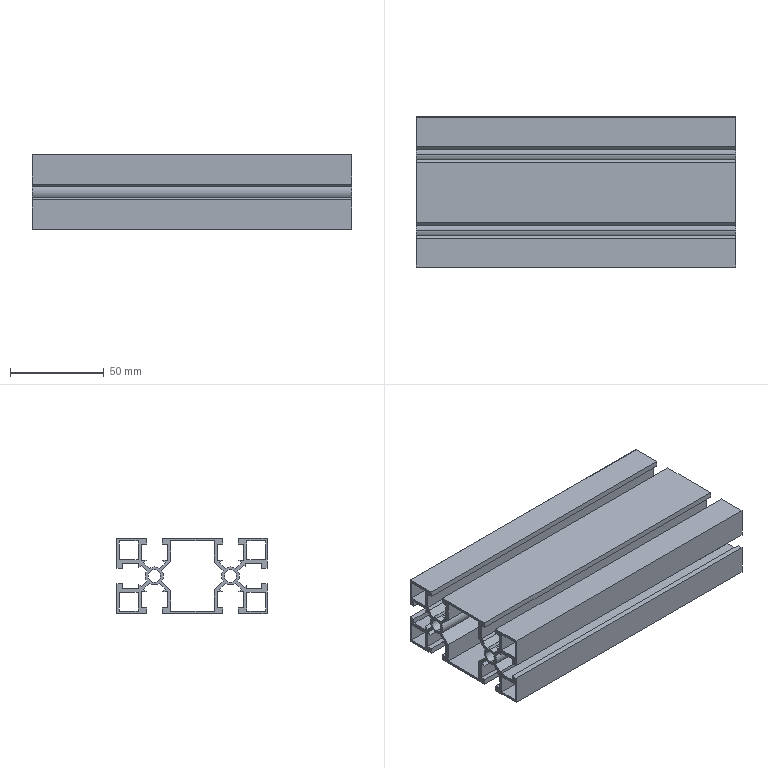Part | 1 solid | 126 faces | box 170 x 80 x 40 mm | volume 117910 mm3 | plane 110 | cylinder 16 | commonest cylinder face diameters 9.6 x10 6.6 x4 0.6 x2